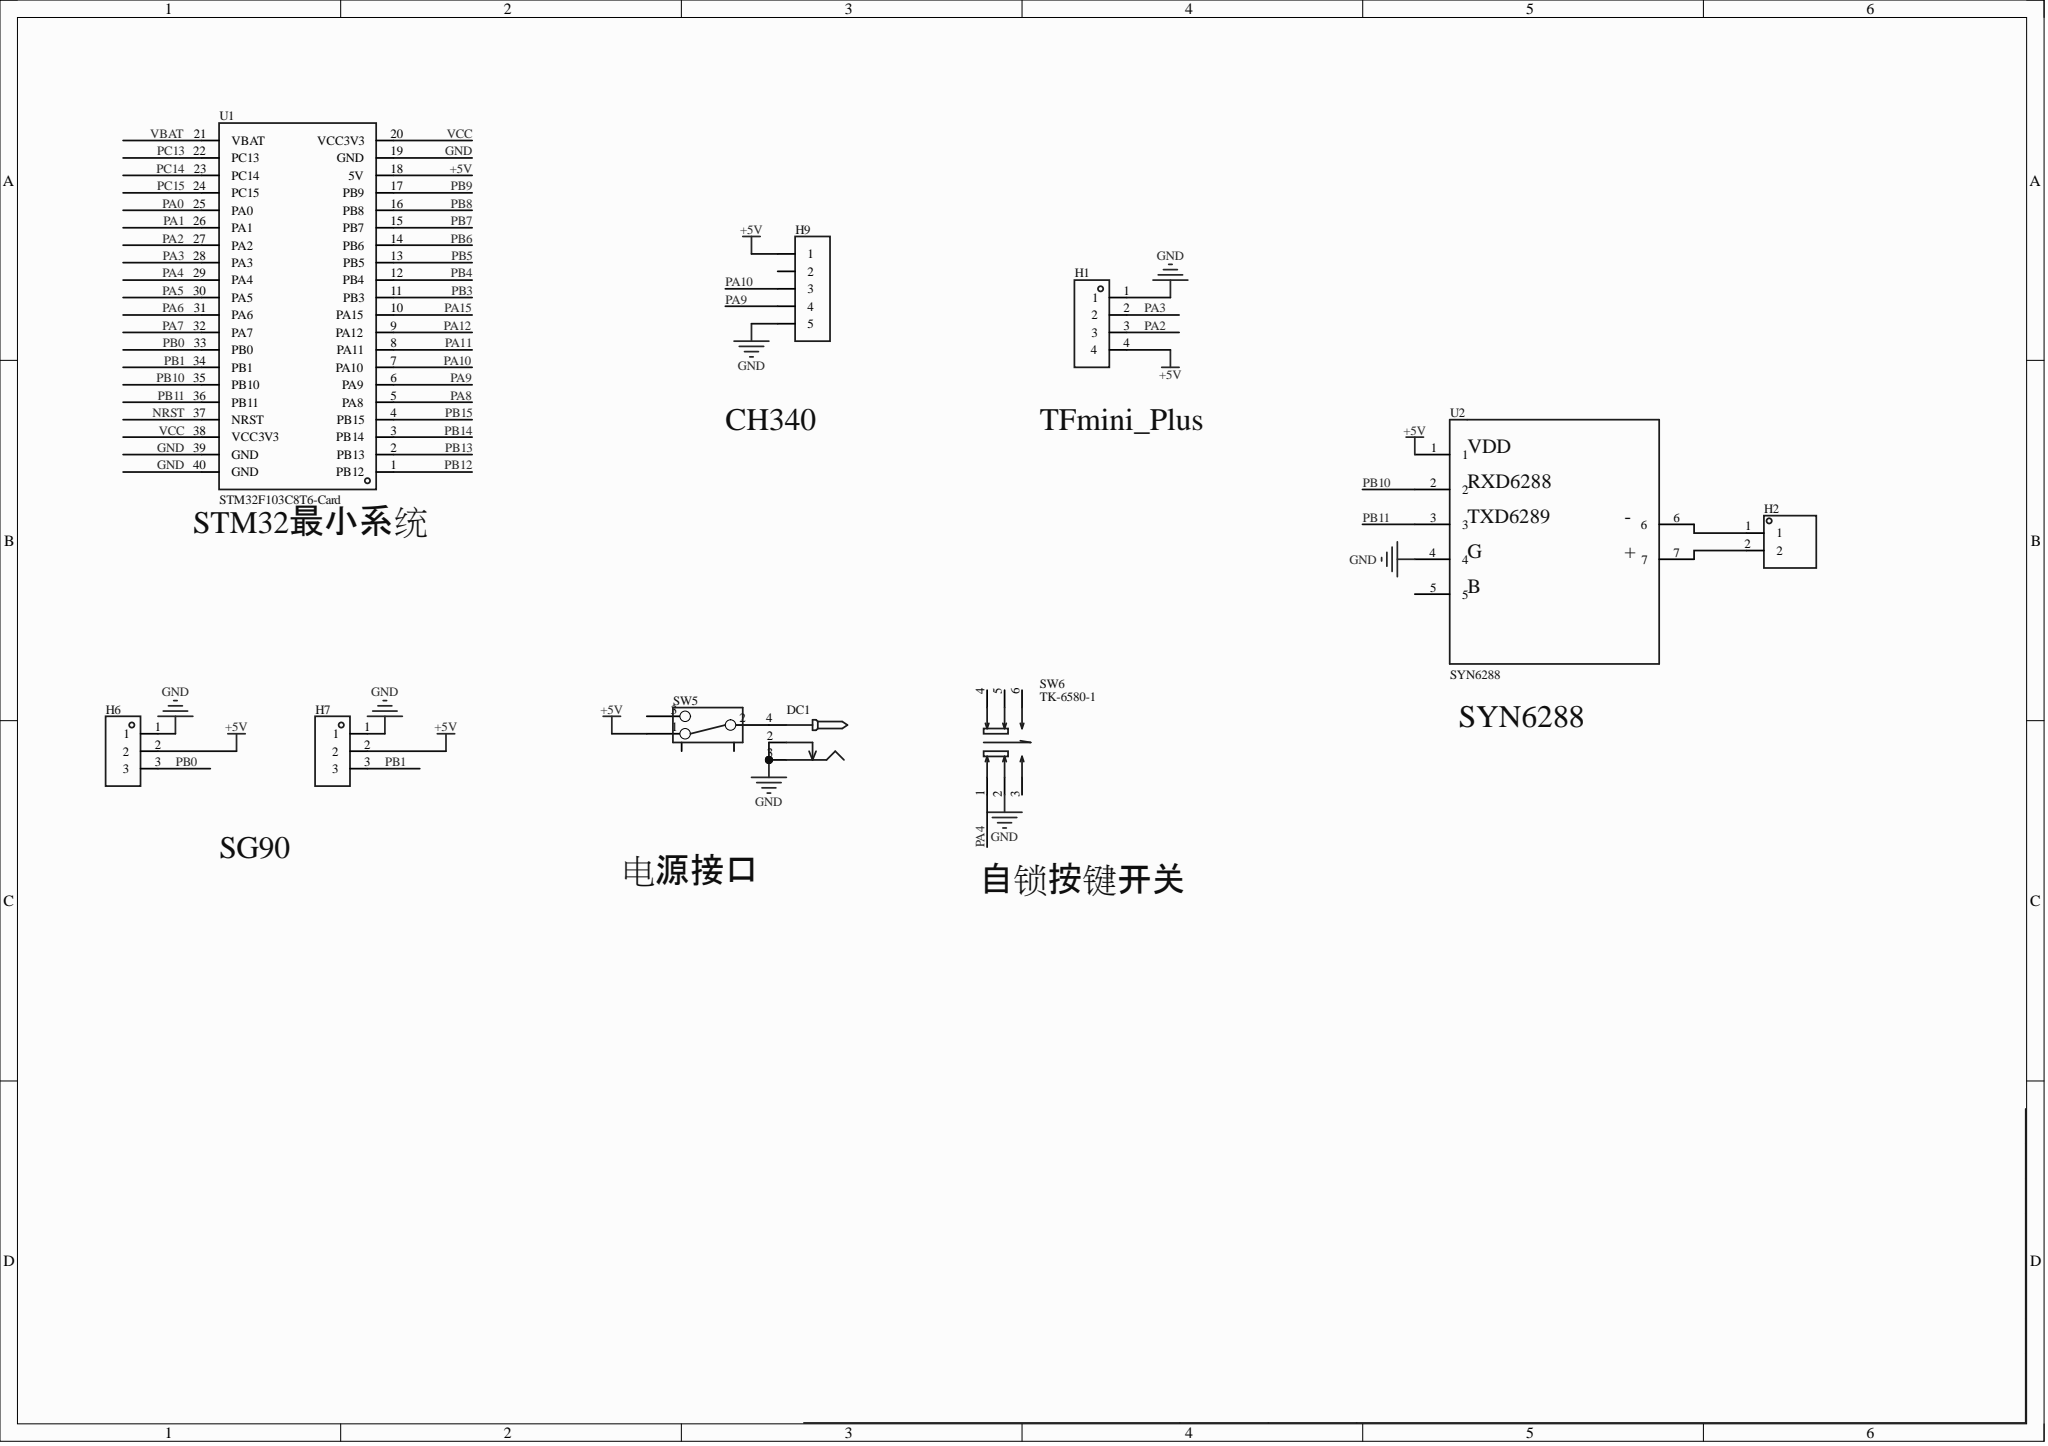Circuit board | Altium Designer | 10 parts | 15 nets
Bill of materials:
Comment,Description,Designator,Footprint,LibRef,Quantity
"","","DC1","DC-2.0","DC-005_2.0","1"
"","","H1","HDR-TH_4P-P2.54-V-F","HDR-F_2.54_1x4P","1"
"","","H2","HDR-TH_2P-P2.54-V-M-1","HDR-M_2.54_1x2P","1"
"","","H6, H7","HDR-TH_3P-P2.54-V-F","HDR-F_2.54_1x3P","2"
"","","H9","HDR-TH_5P-P2.54-V-F","HDR-F_2.54_1x5P","1"
"","","SW5","拨动开关","拨动开关_正","1"
"TK-6580-1","","SW6","SW-TH_TK-6580-1","TK-6580-1","1"
"STM32F103C8T6-Card","","U1","CONN-TH_L53.3-W22.9_STM32F103C8T6-CARD","STM32F103C8T6-Card","1"
"SYN6288","","U2","SYN6288","SYN6288","1"
Netlist (Protel format):
[
DC1
DC-2.0




]
[
H1
HDR-TH_4P-P2.54-V-F




]
[
H2
HDR-TH_2P-P2.54-V-M-1




]
[
H6
HDR-TH_3P-P2.54-V-F




]
[
H7
HDR-TH_3P-P2.54-V-F




]
[
H9
HDR-TH_5P-P2.54-V-F




]
[
SW5
拨动开关




]
[
SW6
SW-TH_TK-6580-1
TK-6580-1



]
[
U1
CONN-TH_L53.3-W22.9_STM32F103C8T6-CARD
STM32F103C8T6-Card



]
[
U2
SYN6288
SYN6288



]
(
VCC
U1-20
U1-38
)
(
PB11
U1-36
U2-3
)
(
PB10
U1-35
U2-2
)
(
PB1
H7-3
U1-34
)
(
PB0
H6-3
U1-33
)
(
PA10
H9-3
U1-7
)
(
PA9
H9-4
U1-6
)
(
PA4
SW6-1
U1-29
)
(
PA3
H1-2
U1-28
)
(
PA2
H1-3
U1-27
)
(
NetH2_2
H2-2
U2-7
)
(
NetH2_1
H2-1
U2-6
)
(
NetDC1_4
DC1-4
SW5-2
)
(
GND
DC1-2
DC1-3
H1-1
H6-1
H7-1
H9-5
SW6-2
U1-19
U1-39
U1-40
U2-4
)
(
+5V
H1-4
H6-2
H7-2
H9-1
SW5-1
U1-18
U2-1
)